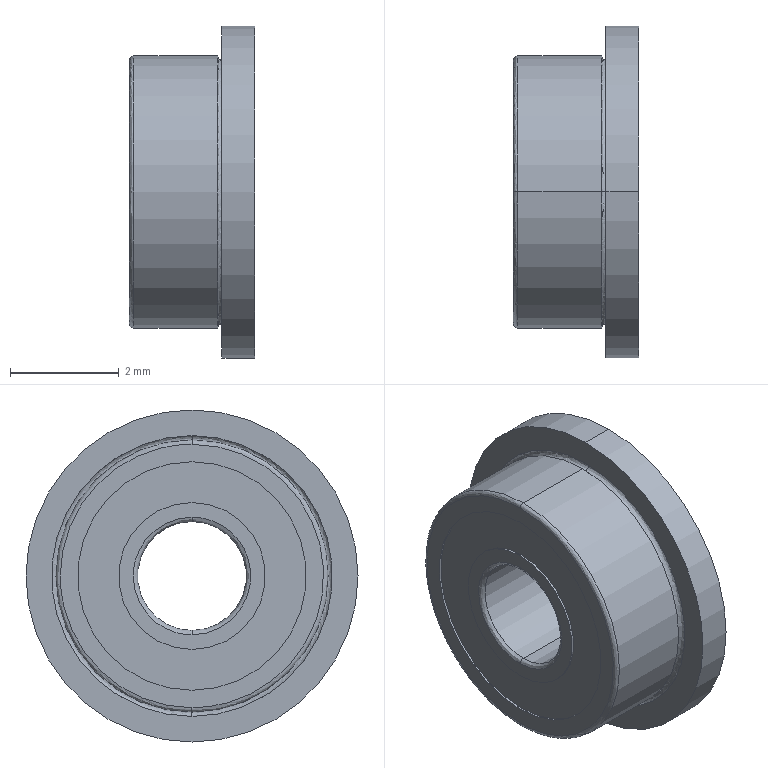Part | SolidWorks | features BaseBody 1 | 1 solid | 29 faces | box 2.3 x 6.1 x 6.1 mm | volume 42.794 mm3 | cylinder 14 | spline 8 | plane 7 | commonest cylinder face diameters 2.7 x4 4.2 x4 2 x2 5 x2 6.1 x2
STEP:
#1=CARTESIAN_POINT('',(1.7,0.,-2.58));
#2=VERTEX_POINT('',#1);
#3=CARTESIAN_POINT('',(1.7,0.,2.58));
#4=VERTEX_POINT('',#3);
#5=CARTESIAN_POINT('',(1.7,0.,0.));
#6=DIRECTION('',(1.,0.,0.));
#7=DIRECTION('',(0.,0.,1.));
#8=AXIS2_PLACEMENT_3D('',#5,#6,#7);
#9=CIRCLE('',#8,2.58);
#10=EDGE_CURVE('',#2,#4,#9,.T.);
#11=ORIENTED_EDGE('',*,*,#10,.F.);
#12=CARTESIAN_POINT('',(1.62,0.,-2.5));
#13=VERTEX_POINT('',#12);
#14=CARTESIAN_POINT('',(1.7,0.,-2.5));
#15=DIRECTION('',(0.,-1.,0.));
#16=DIRECTION('',(0.,0.,-1.));
#17=AXIS2_PLACEMENT_3D('',#14,#15,#16);
#18=CIRCLE('',#17,0.08);
#19=EDGE_CURVE('',#2,#13,#18,.T.);
#20=ORIENTED_EDGE('',*,*,#19,.T.);
#21=CARTESIAN_POINT('',(1.62,0.,2.5));
#22=VERTEX_POINT('',#21);
#23=CARTESIAN_POINT('',(1.62,0.,0.));
#24=DIRECTION('',(-1.,0.,0.));
#25=DIRECTION('',(0.,0.,1.));
#26=AXIS2_PLACEMENT_3D('',#23,#24,#25);
#27=CIRCLE('',#26,2.5);
#28=EDGE_CURVE('',#22,#13,#27,.T.);
#29=ORIENTED_EDGE('',*,*,#28,.F.);
#30=CARTESIAN_POINT('',(1.7,0.,2.5));
#31=DIRECTION('',(0.,1.,0.));
#32=DIRECTION('',(0.,0.,1.));
#33=AXIS2_PLACEMENT_3D('',#30,#31,#32);
#34=CIRCLE('',#33,0.08);
#35=EDGE_CURVE('',#4,#22,#34,.T.);
#36=ORIENTED_EDGE('',*,*,#35,.F.);
#37=EDGE_LOOP('',(#11,#20,#29,#36));
#38=FACE_OUTER_BOUND('',#37,.T.);
#39=CARTESIAN_POINT('',(1.7,0.,2.58));
#40=CARTESIAN_POINT('',(1.7,5.16,2.58));
#41=CARTESIAN_POINT('',(1.7,5.16,-2.58));
#42=CARTESIAN_POINT('',(1.7,0.,-2.58));
#43=CARTESIAN_POINT('',(1.784,0.,2.58));
#44=CARTESIAN_POINT('',(1.784,5.16,2.58));
#45=CARTESIAN_POINT('',(1.784,5.16,-2.58));
#46=CARTESIAN_POINT('',(1.784,0.,-2.58));
#47=CARTESIAN_POINT('',(1.816,0.,2.503));
#48=CARTESIAN_POINT('',(1.816,5.005,2.503));
#49=CARTESIAN_POINT('',(1.816,5.005,-2.503));
#50=CARTESIAN_POINT('',(1.816,0.,-2.503));
#51=CARTESIAN_POINT('',(1.757,0.,2.443));
#52=CARTESIAN_POINT('',(1.757,4.887,2.443));
#53=CARTESIAN_POINT('',(1.757,4.887,-2.443));
#54=CARTESIAN_POINT('',(1.757,0.,-2.443));
#55=CARTESIAN_POINT('',(1.697,0.,2.384));
#56=CARTESIAN_POINT('',(1.697,4.768,2.384));
#57=CARTESIAN_POINT('',(1.697,4.768,-2.384));
#58=CARTESIAN_POINT('',(1.697,0.,-2.384));
#59=CARTESIAN_POINT('',(1.62,0.,2.416));
#60=CARTESIAN_POINT('',(1.62,4.833,2.416));
#61=CARTESIAN_POINT('',(1.62,4.833,-2.416));
#62=CARTESIAN_POINT('',(1.62,0.,-2.416));
#63=CARTESIAN_POINT('',(1.62,0.,2.5));
#64=CARTESIAN_POINT('',(1.62,5.,2.5));
#65=CARTESIAN_POINT('',(1.62,5.,-2.5));
#66=CARTESIAN_POINT('',(1.62,0.,-2.5));
#67=(BOUNDED_SURFACE()B_SPLINE_SURFACE(3,3,((#39,#40,#41,#42),(#43,#44,#45,#46),(#47,#48,#49,#50),(#51,#52,#53,#54),(#55,#56,#57,#58),(#59,#60,#61,#62),(#63,#64,#65,#66)),.UNSPECIFIED.,.F.,.F.,.T.)B_SPLINE_SURFACE_WITH_KNOTS((4,3,4),(4,4),(0.,0.5,1.),(0.,1.),.UNSPECIFIED.)GEOMETRIC_REPRESENTATION_ITEM()RATIONAL_B_SPLINE_SURFACE(((1.,0.3333,0.3333,1.),(0.5885,0.1962,0.1962,0.5885),(0.5885,0.1962,0.1962,0.5885),(1.,0.3333,0.3333,1.),(0.5885,0.1962,0.1962,0.5885),(0.5885,0.1962,0.1962,0.5885),(1.,0.3333,0.3333,1.)))REPRESENTATION_ITEM('')SURFACE());
#68=ADVANCED_FACE('',(#38),#67,.F.);
#69=CARTESIAN_POINT('',(2.3,0.,-1.08));
#70=VERTEX_POINT('',#69);
#71=CARTESIAN_POINT('',(2.3,0.,1.08));
#72=VERTEX_POINT('',#71);
#73=CARTESIAN_POINT('',(2.3,0.,-1.08));
#74=CARTESIAN_POINT('',(2.3,-0.06875,-1.08));
#75=CARTESIAN_POINT('',(2.3,-0.17,-1.07));
#76=CARTESIAN_POINT('',(2.3,-0.2849,-1.043));
#77=CARTESIAN_POINT('',(2.3,-0.3334,-1.027));
#78=CARTESIAN_POINT('',(2.3,-0.3656,-1.016));
#79=CARTESIAN_POINT('',(2.3,-0.3802,-1.011));
#80=CARTESIAN_POINT('',(2.3,-0.5359,-0.9495));
#81=CARTESIAN_POINT('',(2.3,-0.6584,-0.8688));
#82=CARTESIAN_POINT('',(2.3,-0.8163,-0.7111));
#83=CARTESIAN_POINT('',(2.3,-0.8858,-0.6259));
#84=CARTESIAN_POINT('',(2.3,-0.9505,-0.5154));
#85=CARTESIAN_POINT('',(2.3,-0.9747,-0.4657));
#86=CARTESIAN_POINT('',(2.3,-0.99,-0.432));
#87=CARTESIAN_POINT('',(2.3,-0.9979,-0.4135));
#88=CARTESIAN_POINT('',(2.3,-1.055,-0.2702));
#89=CARTESIAN_POINT('',(2.3,-1.08,-0.137));
#90=CARTESIAN_POINT('',(2.3,-1.08,0.06849));
#91=CARTESIAN_POINT('',(2.3,-1.071,0.1696));
#92=CARTESIAN_POINT('',(2.3,-1.043,0.2845));
#93=CARTESIAN_POINT('',(2.3,-1.028,0.3332));
#94=CARTESIAN_POINT('',(2.3,-1.016,0.3655));
#95=CARTESIAN_POINT('',(2.3,-1.011,0.3802));
#96=CARTESIAN_POINT('',(2.3,-0.9495,0.5359));
#97=CARTESIAN_POINT('',(2.3,-0.8688,0.6584));
#98=CARTESIAN_POINT('',(2.3,-0.7111,0.8163));
#99=CARTESIAN_POINT('',(2.3,-0.6259,0.8858));
#100=CARTESIAN_POINT('',(2.3,-0.5154,0.9505));
#101=CARTESIAN_POINT('',(2.3,-0.4657,0.9747));
#102=CARTESIAN_POINT('',(2.3,-0.432,0.99));
#103=CARTESIAN_POINT('',(2.3,-0.4134,0.9979));
#104=CARTESIAN_POINT('',(2.3,-0.2704,1.055));
#105=CARTESIAN_POINT('',(2.3,-0.1379,1.08));
#106=CARTESIAN_POINT('',(2.3,0.,1.08));
#107=B_SPLINE_CURVE_WITH_KNOTS('',3,(#73,#74,#75,#76,#77,#78,#79,#80,#81,#82,#83,#84,#85,#86,#87,#88,#89,#90,#91,#92,#93,#94,#95,#96,#97,#98,#99,#100,#101,#102,#103,#104,#105,#106),.UNSPECIFIED.,.F.,.F.,(4,1,1,2,2,2,1,1,2,2,2,1,1,2,2,2,1,1,2,2,4),(0.,0.0625,0.09375,0.1094,0.125,0.25,0.3125,0.3438,0.3594,0.375,0.5,0.5625,0.5938,0.6094,0.625,0.75,0.8125,0.8438,0.8594,0.875,1.),.UNSPECIFIED.);
#108=EDGE_CURVE('',#70,#72,#107,.T.);
#109=ORIENTED_EDGE('',*,*,#108,.F.);
#110=CARTESIAN_POINT('',(2.22,0.,-1.));
#111=VERTEX_POINT('',#110);
#112=CARTESIAN_POINT('',(2.22,0.,-1.08));
#113=DIRECTION('',(0.,-1.,0.));
#114=DIRECTION('',(0.,0.,-1.));
#115=AXIS2_PLACEMENT_3D('',#112,#113,#114);
#116=CIRCLE('',#115,0.08);
#117=EDGE_CURVE('',#70,#111,#116,.T.);
#118=ORIENTED_EDGE('',*,*,#117,.T.);
#119=CARTESIAN_POINT('',(2.22,0.,1.));
#120=VERTEX_POINT('',#119);
#121=CARTESIAN_POINT('',(2.22,0.,0.));
#122=DIRECTION('',(-1.,0.,0.));
#123=DIRECTION('',(0.,0.,1.));
#124=AXIS2_PLACEMENT_3D('',#121,#122,#123);
#125=CIRCLE('',#124,1.);
#126=EDGE_CURVE('',#111,#120,#125,.T.);
#127=ORIENTED_EDGE('',*,*,#126,.T.);
#128=CARTESIAN_POINT('',(2.22,0.,1.08));
#129=DIRECTION('',(0.,1.,0.));
#130=DIRECTION('',(0.,0.,1.));
#131=AXIS2_PLACEMENT_3D('',#128,#129,#130);
#132=CIRCLE('',#131,0.08);
#133=EDGE_CURVE('',#72,#120,#132,.T.);
#134=ORIENTED_EDGE('',*,*,#133,.F.);
#135=EDGE_LOOP('',(#109,#118,#127,#134));
#136=FACE_OUTER_BOUND('',#135,.T.);
#137=CARTESIAN_POINT('',(2.3,0.,-1.08));
#138=CARTESIAN_POINT('',(2.3,-2.16,-1.08));
#139=CARTESIAN_POINT('',(2.3,-2.16,1.08));
#140=CARTESIAN_POINT('',(2.3,0.,1.08));
#141=CARTESIAN_POINT('',(2.3,0.,-1.033));
#142=CARTESIAN_POINT('',(2.3,-2.066,-1.033));
#143=CARTESIAN_POINT('',(2.3,-2.066,1.033));
#144=CARTESIAN_POINT('',(2.3,0.,1.033));
#145=CARTESIAN_POINT('',(2.267,0.,-1.));
#146=CARTESIAN_POINT('',(2.267,-2.,-1.));
#147=CARTESIAN_POINT('',(2.267,-2.,1.));
#148=CARTESIAN_POINT('',(2.267,0.,1.));
#149=CARTESIAN_POINT('',(2.22,0.,-1.));
#150=CARTESIAN_POINT('',(2.22,-2.,-1.));
#151=CARTESIAN_POINT('',(2.22,-2.,1.));
#152=CARTESIAN_POINT('',(2.22,0.,1.));
#153=(BOUNDED_SURFACE()B_SPLINE_SURFACE(3,3,((#137,#138,#139,#140),(#141,#142,#143,#144),(#145,#146,#147,#148),(#149,#150,#151,#152)),.UNSPECIFIED.,.F.,.F.,.T.)B_SPLINE_SURFACE_WITH_KNOTS((4,4),(4,4),(0.,1.),(0.,1.),.UNSPECIFIED.)GEOMETRIC_REPRESENTATION_ITEM()RATIONAL_B_SPLINE_SURFACE(((1.,0.3333,0.3333,1.),(0.8047,0.2682,0.2682,0.8047),(0.8047,0.2682,0.2682,0.8047),(1.,0.3333,0.3333,1.)))REPRESENTATION_ITEM('')SURFACE());
#154=ADVANCED_FACE('',(#136),#153,.T.);
#155=CARTESIAN_POINT('',(0.,0.,2.42));
#156=VERTEX_POINT('',#155);
#157=CARTESIAN_POINT('',(0.,0.,-2.42));
#158=VERTEX_POINT('',#157);
#159=CARTESIAN_POINT('',(0.,0.,2.42));
#160=CARTESIAN_POINT('',(0.,-4.84,2.42));
#161=CARTESIAN_POINT('',(0.,-4.84,-2.42));
#162=CARTESIAN_POINT('',(0.,0.,-2.42));
#163=(BOUNDED_CURVE()B_SPLINE_CURVE(3,(#159,#160,#161,#162),.UNSPECIFIED.,.F.,.F.)B_SPLINE_CURVE_WITH_KNOTS((4,4),(0.,1.),.UNSPECIFIED.)CURVE()GEOMETRIC_REPRESENTATION_ITEM()RATIONAL_B_SPLINE_CURVE((1.,0.3333,0.3333,1.))REPRESENTATION_ITEM(''));
#164=EDGE_CURVE('',#156,#158,#163,.T.);
#165=ORIENTED_EDGE('',*,*,#164,.T.);
#166=CARTESIAN_POINT('',(0.08,0.,-2.5));
#167=VERTEX_POINT('',#166);
#168=CARTESIAN_POINT('',(0.08,0.,-2.42));
#169=DIRECTION('',(0.,-1.,0.));
#170=DIRECTION('',(0.,0.,-1.));
#171=AXIS2_PLACEMENT_3D('',#168,#169,#170);
#172=CIRCLE('',#171,0.08);
#173=EDGE_CURVE('',#158,#167,#172,.T.);
#174=ORIENTED_EDGE('',*,*,#173,.T.);
#175=CARTESIAN_POINT('',(0.08,0.,2.5));
#176=VERTEX_POINT('',#175);
#177=CARTESIAN_POINT('',(0.08,0.,0.));
#178=DIRECTION('',(1.,0.,0.));
#179=DIRECTION('',(0.,0.,-1.));
#180=AXIS2_PLACEMENT_3D('',#177,#178,#179);
#181=CIRCLE('',#180,2.5);
#182=EDGE_CURVE('',#176,#167,#181,.T.);
#183=ORIENTED_EDGE('',*,*,#182,.F.);
#184=CARTESIAN_POINT('',(0.08,0.,2.42));
#185=DIRECTION('',(0.,1.,0.));
#186=DIRECTION('',(0.,0.,1.));
#187=AXIS2_PLACEMENT_3D('',#184,#185,#186);
#188=CIRCLE('',#187,0.08);
#189=EDGE_CURVE('',#156,#176,#188,.T.);
#190=ORIENTED_EDGE('',*,*,#189,.F.);
#191=EDGE_LOOP('',(#165,#174,#183,#190));
#192=FACE_OUTER_BOUND('',#191,.T.);
#193=CARTESIAN_POINT('',(0.,0.,-2.42));
#194=CARTESIAN_POINT('',(0.,-4.84,-2.42));
#195=CARTESIAN_POINT('',(0.,-4.84,2.42));
#196=CARTESIAN_POINT('',(0.,0.,2.42));
#197=CARTESIAN_POINT('',(0.,0.,-2.467));
#198=CARTESIAN_POINT('',(0.,-4.934,-2.467));
#199=CARTESIAN_POINT('',(0.,-4.934,2.467));
#200=CARTESIAN_POINT('',(0.,0.,2.467));
#201=CARTESIAN_POINT('',(0.03314,0.,-2.5));
#202=CARTESIAN_POINT('',(0.03314,-5.,-2.5));
#203=CARTESIAN_POINT('',(0.03314,-5.,2.5));
#204=CARTESIAN_POINT('',(0.03314,0.,2.5));
#205=CARTESIAN_POINT('',(0.08,0.,-2.5));
#206=CARTESIAN_POINT('',(0.08,-5.,-2.5));
#207=CARTESIAN_POINT('',(0.08,-5.,2.5));
#208=CARTESIAN_POINT('',(0.08,0.,2.5));
#209=(BOUNDED_SURFACE()B_SPLINE_SURFACE(3,3,((#193,#194,#195,#196),(#197,#198,#199,#200),(#201,#202,#203,#204),(#205,#206,#207,#208)),.UNSPECIFIED.,.F.,.F.,.T.)B_SPLINE_SURFACE_WITH_KNOTS((4,4),(4,4),(0.,1.),(0.,1.),.UNSPECIFIED.)GEOMETRIC_REPRESENTATION_ITEM()RATIONAL_B_SPLINE_SURFACE(((1.,0.3333,0.3333,1.),(0.8047,0.2682,0.2682,0.8047),(0.8047,0.2682,0.2682,0.8047),(1.,0.3333,0.3333,1.)))REPRESENTATION_ITEM('')SURFACE());
#210=ADVANCED_FACE('',(#192),#209,.T.);
#211=CARTESIAN_POINT('',(0.08,0.,1.));
#212=VERTEX_POINT('',#211);
#213=CARTESIAN_POINT('',(0.08,0.,-1.));
#214=VERTEX_POINT('',#213);
#215=CARTESIAN_POINT('',(0.08,0.,0.));
#216=DIRECTION('',(1.,0.,0.));
#217=DIRECTION('',(0.,0.,-1.));
#218=AXIS2_PLACEMENT_3D('',#215,#216,#217);
#219=CIRCLE('',#218,1.);
#220=EDGE_CURVE('',#212,#214,#219,.T.);
#221=ORIENTED_EDGE('',*,*,#220,.T.);
#222=CARTESIAN_POINT('',(0.,0.,-1.08));
#223=VERTEX_POINT('',#222);
#224=CARTESIAN_POINT('',(0.08,0.,-1.08));
#225=DIRECTION('',(0.,-1.,0.));
#226=DIRECTION('',(0.,0.,-1.));
#227=AXIS2_PLACEMENT_3D('',#224,#225,#226);
#228=CIRCLE('',#227,0.08);
#229=EDGE_CURVE('',#214,#223,#228,.T.);
#230=ORIENTED_EDGE('',*,*,#229,.T.);
#231=CARTESIAN_POINT('',(0.,0.,1.08));
#232=VERTEX_POINT('',#231);
#233=CARTESIAN_POINT('',(0.,0.,-1.08));
#234=CARTESIAN_POINT('',(0.,-2.16,-1.08));
#235=CARTESIAN_POINT('',(0.,-2.16,1.08));
#236=CARTESIAN_POINT('',(0.,0.,1.08));
#237=(BOUNDED_CURVE()B_SPLINE_CURVE(3,(#233,#234,#235,#236),.UNSPECIFIED.,.F.,.T.)B_SPLINE_CURVE_WITH_KNOTS((4,4),(0.,1.),.UNSPECIFIED.)CURVE()GEOMETRIC_REPRESENTATION_ITEM()RATIONAL_B_SPLINE_CURVE((1.,0.3333,0.3333,1.))REPRESENTATION_ITEM(''));
#238=EDGE_CURVE('',#223,#232,#237,.T.);
#239=ORIENTED_EDGE('',*,*,#238,.T.);
#240=CARTESIAN_POINT('',(0.08,0.,1.08));
#241=DIRECTION('',(0.,1.,0.));
#242=DIRECTION('',(0.,0.,1.));
#243=AXIS2_PLACEMENT_3D('',#240,#241,#242);
#244=CIRCLE('',#243,0.08);
#245=EDGE_CURVE('',#212,#232,#244,.T.);
#246=ORIENTED_EDGE('',*,*,#245,.F.);
#247=EDGE_LOOP('',(#221,#230,#239,#246));
#248=FACE_OUTER_BOUND('',#247,.T.);
#249=CARTESIAN_POINT('',(0.08,0.,-1.));
#250=CARTESIAN_POINT('',(0.08,-2.,-1.));
#251=CARTESIAN_POINT('',(0.08,-2.,1.));
#252=CARTESIAN_POINT('',(0.08,0.,1.));
#253=CARTESIAN_POINT('',(0.03314,0.,-1.));
#254=CARTESIAN_POINT('',(0.03314,-2.,-1.));
#255=CARTESIAN_POINT('',(0.03314,-2.,1.));
#256=CARTESIAN_POINT('',(0.03314,0.,1.));
#257=CARTESIAN_POINT('',(0.,0.,-1.033));
#258=CARTESIAN_POINT('',(0.,-2.066,-1.033));
#259=CARTESIAN_POINT('',(0.,-2.066,1.033));
#260=CARTESIAN_POINT('',(0.,0.,1.033));
#261=CARTESIAN_POINT('',(0.,0.,-1.08));
#262=CARTESIAN_POINT('',(0.,-2.16,-1.08));
#263=CARTESIAN_POINT('',(0.,-2.16,1.08));
#264=CARTESIAN_POINT('',(0.,0.,1.08));
#265=(BOUNDED_SURFACE()B_SPLINE_SURFACE(3,3,((#249,#250,#251,#252),(#253,#254,#255,#256),(#257,#258,#259,#260),(#261,#262,#263,#264)),.UNSPECIFIED.,.F.,.F.,.T.)B_SPLINE_SURFACE_WITH_KNOTS((4,4),(4,4),(0.,1.),(0.,1.),.UNSPECIFIED.)GEOMETRIC_REPRESENTATION_ITEM()RATIONAL_B_SPLINE_SURFACE(((1.,0.3333,0.3333,1.),(0.8047,0.2682,0.2682,0.8047),(0.8047,0.2682,0.2682,0.8047),(1.,0.3333,0.3333,1.)))REPRESENTATION_ITEM('')SURFACE());
#266=ADVANCED_FACE('',(#248),#265,.T.);
#267=CARTESIAN_POINT('',(2.262,0.,2.1));
#268=VERTEX_POINT('',#267);
#269=CARTESIAN_POINT('',(2.262,0.,-2.1));
#270=VERTEX_POINT('',#269);
#271=CARTESIAN_POINT('',(2.262,0.,0.));
#272=DIRECTION('',(1.,0.,0.));
#273=DIRECTION('',(0.,0.,-1.));
#274=AXIS2_PLACEMENT_3D('',#271,#272,#273);
#275=CIRCLE('',#274,2.1);
#276=EDGE_CURVE('',#268,#270,#275,.T.);
#277=ORIENTED_EDGE('',*,*,#276,.F.);
#278=CARTESIAN_POINT('',(2.3,0.,2.1));
#279=VERTEX_POINT('',#278);
#280=CARTESIAN_POINT('',(2.281,0.,2.1));
#281=DIRECTION('',(1.,0.,0.));
#282=VECTOR('',#281,1000.);
#283=LINE('',#280,#282);
#284=EDGE_CURVE('',#268,#279,#283,.T.);
#285=ORIENTED_EDGE('',*,*,#284,.T.);
#286=CARTESIAN_POINT('',(2.3,0.,-2.1));
#287=VERTEX_POINT('',#286);
#288=CARTESIAN_POINT('',(2.3,0.,0.));
#289=DIRECTION('',(-1.,0.,0.));
#290=DIRECTION('',(0.,0.,-1.));
#291=AXIS2_PLACEMENT_3D('',#288,#289,#290);
#292=CIRCLE('',#291,2.1);
#293=EDGE_CURVE('',#287,#279,#292,.T.);
#294=ORIENTED_EDGE('',*,*,#293,.F.);
#295=CARTESIAN_POINT('',(2.281,0.,-2.1));
#296=DIRECTION('',(1.,0.,0.));
#297=VECTOR('',#296,1000.);
#298=LINE('',#295,#297);
#299=EDGE_CURVE('',#270,#287,#298,.T.);
#300=ORIENTED_EDGE('',*,*,#299,.F.);
#301=EDGE_LOOP('',(#277,#285,#294,#300));
#302=FACE_OUTER_BOUND('',#301,.T.);
#303=CARTESIAN_POINT('',(2.281,0.,0.));
#304=DIRECTION('',(1.,0.,0.));
#305=DIRECTION('',(0.,0.,-1.));
#306=AXIS2_PLACEMENT_3D('',#303,#304,#305);
#307=CYLINDRICAL_SURFACE('',#306,2.1);
#308=ADVANCED_FACE('',(#302),#307,.F.);
#309=CARTESIAN_POINT('',(1.7,0.,-3.05));
#310=VERTEX_POINT('',#309);
#311=CARTESIAN_POINT('',(1.7,0.,3.05));
#312=VERTEX_POINT('',#311);
#313=CARTESIAN_POINT('',(1.7,0.,0.));
#314=DIRECTION('',(1.,0.,0.));
#315=DIRECTION('',(0.,0.,-1.));
#316=AXIS2_PLACEMENT_3D('',#313,#314,#315);
#317=CIRCLE('',#316,3.05);
#318=EDGE_CURVE('',#310,#312,#317,.T.);
#319=ORIENTED_EDGE('',*,*,#318,.T.);
#320=CARTESIAN_POINT('',(2.3,0.,3.05));
#321=VERTEX_POINT('',#320);
#322=CARTESIAN_POINT('',(2.,0.,3.05));
#323=DIRECTION('',(1.,0.,0.));
#324=VECTOR('',#323,1000.);
#325=LINE('',#322,#324);
#326=EDGE_CURVE('',#312,#321,#325,.T.);
#327=ORIENTED_EDGE('',*,*,#326,.T.);
#328=CARTESIAN_POINT('',(2.3,0.,-3.05));
#329=VERTEX_POINT('',#328);
#330=CARTESIAN_POINT('',(2.3,0.,0.));
#331=DIRECTION('',(1.,0.,0.));
#332=DIRECTION('',(0.,0.,-1.));
#333=AXIS2_PLACEMENT_3D('',#330,#331,#332);
#334=CIRCLE('',#333,3.05);
#335=EDGE_CURVE('',#329,#321,#334,.T.);
#336=ORIENTED_EDGE('',*,*,#335,.F.);
#337=CARTESIAN_POINT('',(2.,0.,-3.05));
#338=DIRECTION('',(1.,0.,0.));
#339=VECTOR('',#338,1000.);
#340=LINE('',#337,#339);
#341=EDGE_CURVE('',#310,#329,#340,.T.);
#342=ORIENTED_EDGE('',*,*,#341,.F.);
#343=EDGE_LOOP('',(#319,#327,#336,#342));
#344=FACE_OUTER_BOUND('',#343,.T.);
#345=CARTESIAN_POINT('',(2.,0.,0.));
#346=DIRECTION('',(1.,0.,0.));
#347=DIRECTION('',(0.,0.,-1.));
#348=AXIS2_PLACEMENT_3D('',#345,#346,#347);
#349=CYLINDRICAL_SURFACE('',#348,3.05);
#350=ADVANCED_FACE('',(#344),#349,.T.);
#351=CARTESIAN_POINT('',(2.262,0.,1.35));
#352=VERTEX_POINT('',#351);
#353=CARTESIAN_POINT('',(2.262,0.,-1.35));
#354=VERTEX_POINT('',#353);
#355=CARTESIAN_POINT('',(2.262,0.,0.));
#356=DIRECTION('',(-1.,0.,0.));
#357=DIRECTION('',(0.,0.,-1.));
#358=AXIS2_PLACEMENT_3D('',#355,#356,#357);
#359=CIRCLE('',#358,1.35);
#360=EDGE_CURVE('',#352,#354,#359,.T.);
#361=ORIENTED_EDGE('',*,*,#360,.F.);
#362=CARTESIAN_POINT('',(2.3,0.,1.35));
#363=VERTEX_POINT('',#362);
#364=CARTESIAN_POINT('',(2.281,0.,1.35));
#365=DIRECTION('',(1.,0.,0.));
#366=VECTOR('',#365,1000.);
#367=LINE('',#364,#366);
#368=EDGE_CURVE('',#352,#363,#367,.T.);
#369=ORIENTED_EDGE('',*,*,#368,.T.);
#370=CARTESIAN_POINT('',(2.3,0.,-1.35));
#371=VERTEX_POINT('',#370);
#372=CARTESIAN_POINT('',(2.3,0.,0.));
#373=DIRECTION('',(-1.,0.,0.));
#374=DIRECTION('',(0.,0.,-1.));
#375=AXIS2_PLACEMENT_3D('',#372,#373,#374);
#376=CIRCLE('',#375,1.35);
#377=EDGE_CURVE('',#363,#371,#376,.T.);
#378=ORIENTED_EDGE('',*,*,#377,.T.);
#379=CARTESIAN_POINT('',(2.281,0.,-1.35));
#380=DIRECTION('',(1.,0.,0.));
#381=VECTOR('',#380,1000.);
#382=LINE('',#379,#381);
#383=EDGE_CURVE('',#354,#371,#382,.T.);
#384=ORIENTED_EDGE('',*,*,#383,.F.);
#385=EDGE_LOOP('',(#361,#369,#378,#384));
#386=FACE_OUTER_BOUND('',#385,.T.);
#387=CARTESIAN_POINT('',(2.281,0.,0.));
#388=DIRECTION('',(1.,0.,0.));
#389=DIRECTION('',(0.,0.,-1.));
#390=AXIS2_PLACEMENT_3D('',#387,#388,#389);
#391=CYLINDRICAL_SURFACE('',#390,1.35);
#392=ADVANCED_FACE('',(#386),#391,.T.);
#393=CARTESIAN_POINT('',(0.08,0.,0.));
#394=DIRECTION('',(1.,0.,0.));
#395=DIRECTION('',(0.,0.,-1.));
#396=AXIS2_PLACEMENT_3D('',#393,#394,#395);
#397=CIRCLE('',#396,2.5);
#398=EDGE_CURVE('',#167,#176,#397,.T.);
#399=ORIENTED_EDGE('',*,*,#398,.T.);
#400=CARTESIAN_POINT('',(0.85,0.,2.5));
#401=DIRECTION('',(1.,0.,0.));
#402=VECTOR('',#401,1000.);
#403=LINE('',#400,#402);
#404=EDGE_CURVE('',#176,#22,#403,.T.);
#405=ORIENTED_EDGE('',*,*,#404,.T.);
#406=ORIENTED_EDGE('',*,*,#28,.T.);
#407=CARTESIAN_POINT('',(0.85,0.,-2.5));
#408=DIRECTION('',(1.,0.,0.));
#409=VECTOR('',#408,1000.);
#410=LINE('',#407,#409);
#411=EDGE_CURVE('',#167,#13,#410,.T.);
#412=ORIENTED_EDGE('',*,*,#411,.F.);
#413=EDGE_LOOP('',(#399,#405,#406,#412));
#414=FACE_OUTER_BOUND('',#413,.T.);
#415=CARTESIAN_POINT('',(0.85,0.,0.));
#416=DIRECTION('',(1.,0.,0.));
#417=DIRECTION('',(0.,0.,-1.));
#418=AXIS2_PLACEMENT_3D('',#415,#416,#417);
#419=CYLINDRICAL_SURFACE('',#418,2.5);
#420=ADVANCED_FACE('',(#414),#419,.T.);
#421=ORIENTED_EDGE('',*,*,#220,.F.);
#422=CARTESIAN_POINT('',(1.15,0.,1.));
#423=DIRECTION('',(1.,0.,0.));
#424=VECTOR('',#423,1000.);
#425=LINE('',#422,#424);
#426=EDGE_CURVE('',#212,#120,#425,.T.);
#427=ORIENTED_EDGE('',*,*,#426,.T.);
#428=ORIENTED_EDGE('',*,*,#126,.F.);
#429=CARTESIAN_POINT('',(1.15,0.,-1.));
#430=DIRECTION('',(1.,0.,0.));
#431=VECTOR('',#430,1000.);
#432=LINE('',#429,#431);
#433=EDGE_CURVE('',#214,#111,#432,.T.);
#434=ORIENTED_EDGE('',*,*,#433,.F.);
#435=EDGE_LOOP('',(#421,#427,#428,#434));
#436=FACE_OUTER_BOUND('',#435,.T.);
#437=CARTESIAN_POINT('',(1.15,0.,0.));
#438=DIRECTION('',(1.,0.,0.));
#439=DIRECTION('',(0.,0.,-1.));
#440=AXIS2_PLACEMENT_3D('',#437,#438,#439);
#441=CYLINDRICAL_SURFACE('',#440,1.);
#442=ADVANCED_FACE('',(#436),#441,.F.);
#443=CARTESIAN_POINT('',(0.,0.,2.1));
#444=VERTEX_POINT('',#443);
#445=CARTESIAN_POINT('',(0.,0.,-2.1));
#446=VERTEX_POINT('',#445);
#447=CARTESIAN_POINT('',(0.,0.,0.));
#448=DIRECTION('',(1.,0.,0.));
#449=DIRECTION('',(0.,0.,-1.));
#450=AXIS2_PLACEMENT_3D('',#447,#448,#449);
#451=CIRCLE('',#450,2.1);
#452=EDGE_CURVE('',#444,#446,#451,.T.);
#453=ORIENTED_EDGE('',*,*,#452,.F.);
#454=CARTESIAN_POINT('',(0.0382,0.,2.1));
#455=VERTEX_POINT('',#454);
#456=CARTESIAN_POINT('',(0.0191,0.,2.1));
#457=DIRECTION('',(1.,0.,0.));
#458=VECTOR('',#457,1000.);
#459=LINE('',#456,#458);
#460=EDGE_CURVE('',#444,#455,#459,.T.);
#461=ORIENTED_EDGE('',*,*,#460,.T.);
#462=CARTESIAN_POINT('',(0.0382,0.,-2.1));
#463=VERTEX_POINT('',#462);
#464=CARTESIAN_POINT('',(0.0382,0.,0.));
#465=DIRECTION('',(-1.,0.,0.));
#466=DIRECTION('',(0.,0.,-1.));
#467=AXIS2_PLACEMENT_3D('',#464,#465,#466);
#468=CIRCLE('',#467,2.1);
#469=EDGE_CURVE('',#463,#455,#468,.T.);
#470=ORIENTED_EDGE('',*,*,#469,.F.);
#471=CARTESIAN_POINT('',(0.0191,0.,-2.1));
#472=DIRECTION('',(1.,0.,0.));
#473=VECTOR('',#472,1000.);
#474=LINE('',#471,#473);
#475=EDGE_CURVE('',#446,#463,#474,.T.);
#476=ORIENTED_EDGE('',*,*,#475,.F.);
#477=EDGE_LOOP('',(#453,#461,#470,#476));
#478=FACE_OUTER_BOUND('',#477,.T.);
#479=CARTESIAN_POINT('',(0.0191,0.,0.));
#480=DIRECTION('',(1.,0.,0.));
#481=DIRECTION('',(0.,0.,-1.));
#482=AXIS2_PLACEMENT_3D('',#479,#480,#481);
#483=CYLINDRICAL_SURFACE('',#482,2.1);
#484=ADVANCED_FACE('',(#478),#483,.F.);
#485=CARTESIAN_POINT('',(0.,0.,1.35));
#486=VERTEX_POINT('',#485);
#487=CARTESIAN_POINT('',(0.,0.,-1.35));
#488=VERTEX_POINT('',#487);
#489=CARTESIAN_POINT('',(0.,0.,0.));
#490=DIRECTION('',(-1.,0.,0.));
#491=DIRECTION('',(0.,0.,-1.));
#492=AXIS2_PLACEMENT_3D('',#489,#490,#491);
#493=CIRCLE('',#492,1.35);
#494=EDGE_CURVE('',#486,#488,#493,.T.);
#495=ORIENTED_EDGE('',*,*,#494,.F.);
#496=CARTESIAN_POINT('',(0.0382,0.,1.35));
#497=VERTEX_POINT('',#496);
#498=CARTESIAN_POINT('',(0.0191,0.,1.35));
#499=DIRECTION('',(1.,0.,0.));
#500=VECTOR('',#499,1000.);
#501=LINE('',#498,#500);
#502=EDGE_CURVE('',#486,#497,#501,.T.);
#503=ORIENTED_EDGE('',*,*,#502,.T.);
#504=CARTESIAN_POINT('',(0.0382,0.,-1.35));
#505=VERTEX_POINT('',#504);
#506=CARTESIAN_POINT('',(0.0382,0.,0.));
#507=DIRECTION('',(-1.,0.,0.));
#508=DIRECTION('',(0.,0.,-1.));
#509=AXIS2_PLACEMENT_3D('',#506,#507,#508);
#510=CIRCLE('',#509,1.35);
#511=EDGE_CURVE('',#497,#505,#510,.T.);
#512=ORIENTED_EDGE('',*,*,#511,.T.);
#513=CARTESIAN_POINT('',(0.0191,0.,-1.35));
#514=DIRECTION('',(1.,0.,0.));
#515=VECTOR('',#514,1000.);
#516=LINE('',#513,#515);
#517=EDGE_CURVE('',#488,#505,#516,.T.);
#518=ORIENTED_EDGE('',*,*,#517,.F.);
#519=EDGE_LOOP('',(#495,#503,#512,#518));
#520=FACE_OUTER_BOUND('',#519,.T.);
#521=CARTESIAN_POINT('',(0.0191,0.,0.));
#522=DIRECTION('',(1.,0.,0.));
#523=DIRECTION('',(0.,0.,-1.));
#524=AXIS2_PLACEMENT_3D('',#521,#522,#523);
#525=CYLINDRICAL_SURFACE('',#524,1.35);
#526=ADVANCED_FACE('',(#520),#525,.T.);
#527=ORIENTED_EDGE('',*,*,#293,.T.);
#528=CARTESIAN_POINT('',(2.3,0.,0.));
#529=DIRECTION('',(-1.,0.,0.));
#530=DIRECTION('',(0.,0.,-1.));
#531=AXIS2_PLACEMENT_3D('',#528,#529,#530);
#532=CIRCLE('',#531,2.1);
#533=EDGE_CURVE('',#279,#287,#532,.T.);
#534=ORIENTED_EDGE('',*,*,#533,.T.);
#535=EDGE_LOOP('',(#527,#534));
#536=FACE_BOUND('',#535,.T.);
#537=ORIENTED_EDGE('',*,*,#335,.T.);
#538=CARTESIAN_POINT('',(2.3,0.,0.));
#539=DIRECTION('',(1.,0.,0.));
#540=DIRECTION('',(0.,0.,-1.));
#541=AXIS2_PLACEMENT_3D('',#538,#539,#540);
#542=CIRCLE('',#541,3.05);
#543=EDGE_CURVE('',#321,#329,#542,.T.);
#544=ORIENTED_EDGE('',*,*,#543,.T.);
#545=EDGE_LOOP('',(#537,#544));
#546=FACE_OUTER_BOUND('',#545,.T.);
#547=CARTESIAN_POINT('',(2.3,2.575,0.));
#548=DIRECTION('',(1.,0.,0.));
#549=DIRECTION('',(0.,0.,-1.));
#550=AXIS2_PLACEMENT_3D('',#547,#548,#549);
#551=PLANE('',#550);
#552=ADVANCED_FACE('',(#536,#546),#551,.T.);
#553=ORIENTED_EDGE('',*,*,#284,.F.);
#554=CARTESIAN_POINT('',(2.262,0.,0.));
#555=DIRECTION('',(1.,0.,0.));
#556=DIRECTION('',(0.,0.,-1.));
#557=AXIS2_PLACEMENT_3D('',#554,#555,#556);
#558=CIRCLE('',#557,2.1);
#559=EDGE_CURVE('',#270,#268,#558,.T.);
#560=ORIENTED_EDGE('',*,*,#559,.F.);
#561=ORIENTED_EDGE('',*,*,#299,.T.);
#562=ORIENTED_EDGE('',*,*,#533,.F.);
#563=EDGE_LOOP('',(#553,#560,#561,#562));
#564=FACE_OUTER_BOUND('',#563,.T.);
#565=CARTESIAN_POINT('',(2.281,0.,0.));
#566=DIRECTION('',(1.,0.,0.));
#567=DIRECTION('',(0.,0.,-1.));
#568=AXIS2_PLACEMENT_3D('',#565,#566,#567);
#569=CYLINDRICAL_SURFACE('',#568,2.1);
#570=ADVANCED_FACE('',(#564),#569,.F.);
#571=ORIENTED_EDGE('',*,*,#326,.F.);
#572=CARTESIAN_POINT('',(1.7,0.,0.));
#573=DIRECTION('',(1.,0.,0.));
#574=DIRECTION('',(0.,0.,-1.));
#575=AXIS2_PLACEMENT_3D('',#572,#573,#574);
#576=CIRCLE('',#575,3.05);
#577=EDGE_CURVE('',#312,#310,#576,.T.);
#578=ORIENTED_EDGE('',*,*,#577,.T.);
#579=ORIENTED_EDGE('',*,*,#341,.T.);
#580=ORIENTED_EDGE('',*,*,#543,.F.);
#581=EDGE_LOOP('',(#571,#578,#579,#580));
#582=FACE_OUTER_BOUND('',#581,.T.);
#583=CARTESIAN_POINT('',(2.,0.,0.));
#584=DIRECTION('',(1.,0.,0.));
#585=DIRECTION('',(0.,0.,-1.));
#586=AXIS2_PLACEMENT_3D('',#583,#584,#585);
#587=CYLINDRICAL_SURFACE('',#586,3.05);
#588=ADVANCED_FACE('',(#582),#587,.T.);
#589=CARTESIAN_POINT('',(2.262,0.,0.));
#590=DIRECTION('',(-1.,0.,0.));
#591=DIRECTION('',(0.,0.,-1.));
#592=AXIS2_PLACEMENT_3D('',#589,#590,#591);
#593=CIRCLE('',#592,1.35);
#594=EDGE_CURVE('',#354,#352,#593,.T.);
#595=ORIENTED_EDGE('',*,*,#594,.T.);
#596=ORIENTED_EDGE('',*,*,#360,.T.);
#597=EDGE_LOOP('',(#595,#596));
#598=FACE_BOUND('',#597,.T.);
#599=ORIENTED_EDGE('',*,*,#559,.T.);
#600=ORIENTED_EDGE('',*,*,#276,.T.);
#601=EDGE_LOOP('',(#599,#600));
#602=FACE_OUTER_BOUND('',#601,.T.);
#603=CARTESIAN_POINT('',(2.262,1.725,0.));
#604=DIRECTION('',(1.,0.,0.));
#605=DIRECTION('',(0.,0.,-1.));
#606=AXIS2_PLACEMENT_3D('',#603,#604,#605);
#607=PLANE('',#606);
#608=ADVANCED_FACE('',(#598,#602),#607,.T.);
#609=ORIENTED_EDGE('',*,*,#318,.F.);
#610=ORIENTED_EDGE('',*,*,#577,.F.);
#611=EDGE_LOOP('',(#609,#610));
#612=FACE_OUTER_BOUND('',#611,.T.);
#613=CARTESIAN_POINT('',(1.7,0.,0.));
#614=DIRECTION('',(1.,0.,0.));
#615=DIRECTION('',(0.,0.,1.));
#616=AXIS2_PLACEMENT_3D('',#613,#614,#615);
#617=CIRCLE('',#616,2.58);
#618=EDGE_CURVE('',#4,#2,#617,.T.);
#619=ORIENTED_EDGE('',*,*,#618,.T.);
#620=ORIENTED_EDGE('',*,*,#10,.T.);
#621=EDGE_LOOP('',(#619,#620));
#622=FACE_BOUND('',#621,.T.);
#623=CARTESIAN_POINT('',(1.7,2.815,0.));
#624=DIRECTION('',(-1.,0.,0.));
#625=DIRECTION('',(0.,0.,1.));
#626=AXIS2_PLACEMENT_3D('',#623,#624,#625);
#627=PLANE('',#626);
#628=ADVANCED_FACE('',(#612,#622),#627,.T.);
#629=ORIENTED_EDGE('',*,*,#368,.F.);
#630=ORIENTED_EDGE('',*,*,#594,.F.);
#631=ORIENTED_EDGE('',*,*,#383,.T.);
#632=CARTESIAN_POINT('',(2.3,0.,0.));
#633=DIRECTION('',(-1.,0.,0.));
#634=DIRECTION('',(0.,0.,-1.));
#635=AXIS2_PLACEMENT_3D('',#632,#633,#634);
#636=CIRCLE('',#635,1.35);
#637=EDGE_CURVE('',#371,#363,#636,.T.);
#638=ORIENTED_EDGE('',*,*,#637,.T.);
#639=EDGE_LOOP('',(#629,#630,#631,#638));
#640=FACE_OUTER_BOUND('',#639,.T.);
#641=CARTESIAN_POINT('',(2.281,0.,0.));
#642=DIRECTION('',(1.,0.,0.));
#643=DIRECTION('',(0.,0.,-1.));
#644=AXIS2_PLACEMENT_3D('',#641,#642,#643);
#645=CYLINDRICAL_SURFACE('',#644,1.35);
#646=ADVANCED_FACE('',(#640),#645,.T.);
#647=ORIENTED_EDGE('',*,*,#19,.F.);
#648=ORIENTED_EDGE('',*,*,#618,.F.);
#649=ORIENTED_EDGE('',*,*,#35,.T.);
#650=CARTESIAN_POINT('',(1.62,0.,0.));
#651=DIRECTION('',(-1.,0.,0.));
#652=DIRECTION('',(0.,0.,1.));
#653=AXIS2_PLACEMENT_3D('',#650,#651,#652);
#654=CIRCLE('',#653,2.5);
#655=EDGE_CURVE('',#13,#22,#654,.T.);
#656=ORIENTED_EDGE('',*,*,#655,.F.);
#657=EDGE_LOOP('',(#647,#648,#649,#656));
#658=FACE_OUTER_BOUND('',#657,.T.);
#659=CARTESIAN_POINT('',(1.7,0.,-2.58));
#660=CARTESIAN_POINT('',(1.7,-5.16,-2.58));
#661=CARTESIAN_POINT('',(1.7,-5.16,2.58));
#662=CARTESIAN_POINT('',(1.7,0.,2.58));
#663=CARTESIAN_POINT('',(1.784,0.,-2.58));
#664=CARTESIAN_POINT('',(1.784,-5.16,-2.58));
#665=CARTESIAN_POINT('',(1.784,-5.16,2.58));
#666=CARTESIAN_POINT('',(1.784,0.,2.58));
#667=CARTESIAN_POINT('',(1.816,0.,-2.503));
#668=CARTESIAN_POINT('',(1.816,-5.005,-2.503));
#669=CARTESIAN_POINT('',(1.816,-5.005,2.503));
#670=CARTESIAN_POINT('',(1.816,0.,2.503));
#671=CARTESIAN_POINT('',(1.757,0.,-2.443));
#672=CARTESIAN_POINT('',(1.757,-4.887,-2.443));
#673=CARTESIAN_POINT('',(1.757,-4.887,2.443));
#674=CARTESIAN_POINT('',(1.757,0.,2.443));
#675=CARTESIAN_POINT('',(1.697,0.,-2.384));
#676=CARTESIAN_POINT('',(1.697,-4.768,-2.384));
#677=CARTESIAN_POINT('',(1.697,-4.768,2.384));
#678=CARTESIAN_POINT('',(1.697,0.,2.384));
#679=CARTESIAN_POINT('',(1.62,0.,-2.416));
#680=CARTESIAN_POINT('',(1.62,-4.833,-2.416));
#681=CARTESIAN_POINT('',(1.62,-4.833,2.416));
#682=CARTESIAN_POINT('',(1.62,0.,2.416));
#683=CARTESIAN_POINT('',(1.62,0.,-2.5));
#684=CARTESIAN_POINT('',(1.62,-5.,-2.5));
#685=CARTESIAN_POINT('',(1.62,-5.,2.5));
#686=CARTESIAN_POINT('',(1.62,0.,2.5));
#687=(BOUNDED_SURFACE()B_SPLINE_SURFACE(3,3,((#659,#660,#661,#662),(#663,#664,#665,#666),(#667,#668,#669,#670),(#671,#672,#673,#674),(#675,#676,#677,#678),(#679,#680,#681,#682),(#683,#684,#685,#686)),.UNSPECIFIED.,.F.,.F.,.T.)B_SPLINE_SURFACE_WITH_KNOTS((4,3,4),(4,4),(0.,0.5,1.),(0.,1.),.UNSPECIFIED.)GEOMETRIC_REPRESENTATION_ITEM()RATIONAL_B_SPLINE_SURFACE(((1.,0.3333,0.3333,1.),(0.5885,0.1962,0.1962,0.5885),(0.5885,0.1962,0.1962,0.5885),(1.,0.3333,0.3333,1.),(0.5885,0.1962,0.1962,0.5885),(0.5885,0.1962,0.1962,0.5885),(1.,0.3333,0.3333,1.)))REPRESENTATION_ITEM('')SURFACE());
#688=ADVANCED_FACE('',(#658),#687,.F.);
#689=ORIENTED_EDGE('',*,*,#108,.T.);
#690=CARTESIAN_POINT('',(2.3,1.08,0.));
#691=VERTEX_POINT('',#690);
#692=CARTESIAN_POINT('',(2.3,0.,1.08));
#693=CARTESIAN_POINT('',(2.3,0.06875,1.08));
#694=CARTESIAN_POINT('',(2.3,0.17,1.07));
#695=CARTESIAN_POINT('',(2.3,0.2849,1.043));
#696=CARTESIAN_POINT('',(2.3,0.3334,1.027));
#697=CARTESIAN_POINT('',(2.3,0.3656,1.016));
#698=CARTESIAN_POINT('',(2.3,0.3802,1.011));
#699=CARTESIAN_POINT('',(2.3,0.5359,0.9495));
#700=CARTESIAN_POINT('',(2.3,0.6584,0.8688));
#701=CARTESIAN_POINT('',(2.3,0.8163,0.7111));
#702=CARTESIAN_POINT('',(2.3,0.8858,0.6259));
#703=CARTESIAN_POINT('',(2.3,0.9505,0.5154));
#704=CARTESIAN_POINT('',(2.3,0.9747,0.4657));
#705=CARTESIAN_POINT('',(2.3,0.99,0.432));
#706=CARTESIAN_POINT('',(2.3,0.9979,0.4134));
#707=CARTESIAN_POINT('',(2.3,1.055,0.2704));
#708=CARTESIAN_POINT('',(2.3,1.08,0.1379));
#709=CARTESIAN_POINT('',(2.3,1.08,0.));
#710=B_SPLINE_CURVE_WITH_KNOTS('',3,(#692,#693,#694,#695,#696,#697,#698,#699,#700,#701,#702,#703,#704,#705,#706,#707,#708,#709),.UNSPECIFIED.,.F.,.F.,(4,1,1,2,2,2,1,1,2,2,4),(0.,0.125,0.1875,0.2188,0.25,0.5,0.625,0.6875,0.7187,0.75,1.),.UNSPECIFIED.);
#711=EDGE_CURVE('',#72,#691,#710,.T.);
#712=ORIENTED_EDGE('',*,*,#711,.T.);
#713=CARTESIAN_POINT('',(2.3,1.08,0.));
#714=CARTESIAN_POINT('',(2.3,1.08,-0.06875));
#715=CARTESIAN_POINT('',(2.3,1.07,-0.17));
#716=CARTESIAN_POINT('',(2.3,1.043,-0.2849));
#717=CARTESIAN_POINT('',(2.3,1.027,-0.3334));
#718=CARTESIAN_POINT('',(2.3,1.016,-0.3656));
#719=CARTESIAN_POINT('',(2.3,1.011,-0.3802));
#720=CARTESIAN_POINT('',(2.3,0.9495,-0.5359));
#721=CARTESIAN_POINT('',(2.3,0.8688,-0.6584));
#722=CARTESIAN_POINT('',(2.3,0.7111,-0.8163));
#723=CARTESIAN_POINT('',(2.3,0.6259,-0.8858));
#724=CARTESIAN_POINT('',(2.3,0.5154,-0.9505));
#725=CARTESIAN_POINT('',(2.3,0.4657,-0.9747));
#726=CARTESIAN_POINT('',(2.3,0.432,-0.99));
#727=CARTESIAN_POINT('',(2.3,0.4134,-0.9979));
#728=CARTESIAN_POINT('',(2.3,0.2704,-1.055));
#729=CARTESIAN_POINT('',(2.3,0.1379,-1.08));
#730=CARTESIAN_POINT('',(2.3,0.,-1.08));
#731=B_SPLINE_CURVE_WITH_KNOTS('',3,(#713,#714,#715,#716,#717,#718,#719,#720,#721,#722,#723,#724,#725,#726,#727,#728,#729,#730),.UNSPECIFIED.,.F.,.F.,(4,1,1,2,2,2,1,1,2,2,4),(0.,0.125,0.1875,0.2187,0.25,0.5,0.625,0.6875,0.7188,0.75,1.),.UNSPECIFIED.);
#732=EDGE_CURVE('',#691,#70,#731,.T.);
#733=ORIENTED_EDGE('',*,*,#732,.T.);
#734=EDGE_LOOP('',(#689,#712,#733));
#735=FACE_BOUND('',#734,.T.);
#736=ORIENTED_EDGE('',*,*,#637,.F.);
#737=ORIENTED_EDGE('',*,*,#377,.F.);
#738=EDGE_LOOP('',(#736,#737));
#739=FACE_OUTER_BOUND('',#738,.T.);
#740=CARTESIAN_POINT('',(2.3,1.215,0.));
#741=DIRECTION('',(1.,0.,0.));
#742=DIRECTION('',(0.,0.,-1.));
#743=AXIS2_PLACEMENT_3D('',#740,#741,#742);
#744=PLANE('',#743);
#745=ADVANCED_FACE('',(#735,#739),#744,.T.);
#746=ORIENTED_EDGE('',*,*,#117,.F.);
#747=ORIENTED_EDGE('',*,*,#732,.F.);
#748=ORIENTED_EDGE('',*,*,#711,.F.);
#749=ORIENTED_EDGE('',*,*,#133,.T.);
#750=CARTESIAN_POINT('',(2.22,0.,0.));
#751=DIRECTION('',(-1.,0.,0.));
#752=DIRECTION('',(0.,0.,1.));
#753=AXIS2_PLACEMENT_3D('',#750,#751,#752);
#754=CIRCLE('',#753,1.);
#755=EDGE_CURVE('',#120,#111,#754,.T.);
#756=ORIENTED_EDGE('',*,*,#755,.T.);
#757=EDGE_LOOP('',(#746,#747,#748,#749,#756));
#758=FACE_OUTER_BOUND('',#757,.T.);
#759=CARTESIAN_POINT('',(2.3,0.,1.08));
#760=CARTESIAN_POINT('',(2.3,2.16,1.08));
#761=CARTESIAN_POINT('',(2.3,2.16,-1.08));
#762=CARTESIAN_POINT('',(2.3,0.,-1.08));
#763=CARTESIAN_POINT('',(2.3,0.,1.033));
#764=CARTESIAN_POINT('',(2.3,2.066,1.033));
#765=CARTESIAN_POINT('',(2.3,2.066,-1.033));
#766=CARTESIAN_POINT('',(2.3,0.,-1.033));
#767=CARTESIAN_POINT('',(2.267,0.,1.));
#768=CARTESIAN_POINT('',(2.267,2.,1.));
#769=CARTESIAN_POINT('',(2.267,2.,-1.));
#770=CARTESIAN_POINT('',(2.267,0.,-1.));
#771=CARTESIAN_POINT('',(2.22,0.,1.));
#772=CARTESIAN_POINT('',(2.22,2.,1.));
#773=CARTESIAN_POINT('',(2.22,2.,-1.));
#774=CARTESIAN_POINT('',(2.22,0.,-1.));
#775=(BOUNDED_SURFACE()B_SPLINE_SURFACE(3,3,((#759,#760,#761,#762),(#763,#764,#765,#766),(#767,#768,#769,#770),(#771,#772,#773,#774)),.UNSPECIFIED.,.F.,.F.,.F.)B_SPLINE_SURFACE_WITH_KNOTS((4,4),(4,4),(0.,1.),(0.,1.),.UNSPECIFIED.)GEOMETRIC_REPRESENTATION_ITEM()RATIONAL_B_SPLINE_SURFACE(((1.,0.3333,0.3333,1.),(0.8047,0.2682,0.2682,0.8047),(0.8047,0.2682,0.2682,0.8047),(1.,0.3333,0.3333,1.)))REPRESENTATION_ITEM('')SURFACE());
#776=ADVANCED_FACE('',(#758),#775,.T.);
#777=ORIENTED_EDGE('',*,*,#404,.F.);
#778=ORIENTED_EDGE('',*,*,#182,.T.);
#779=ORIENTED_EDGE('',*,*,#411,.T.);
#780=ORIENTED_EDGE('',*,*,#655,.T.);
#781=EDGE_LOOP('',(#777,#778,#779,#780));
#782=FACE_OUTER_BOUND('',#781,.T.);
#783=CARTESIAN_POINT('',(0.85,0.,0.));
#784=DIRECTION('',(1.,0.,0.));
#785=DIRECTION('',(0.,0.,-1.));
#786=AXIS2_PLACEMENT_3D('',#783,#784,#785);
#787=CYLINDRICAL_SURFACE('',#786,2.5);
#788=ADVANCED_FACE('',(#782),#787,.T.);
#789=ORIENTED_EDGE('',*,*,#426,.F.);
#790=CARTESIAN_POINT('',(0.08,0.,0.));
#791=DIRECTION('',(1.,0.,0.));
#792=DIRECTION('',(0.,0.,-1.));
#793=AXIS2_PLACEMENT_3D('',#790,#791,#792);
#794=CIRCLE('',#793,1.);
#795=EDGE_CURVE('',#214,#212,#794,.T.);
#796=ORIENTED_EDGE('',*,*,#795,.F.);
#797=ORIENTED_EDGE('',*,*,#433,.T.);
#798=ORIENTED_EDGE('',*,*,#755,.F.);
#799=EDGE_LOOP('',(#789,#796,#797,#798));
#800=FACE_OUTER_BOUND('',#799,.T.);
#801=CARTESIAN_POINT('',(1.15,0.,0.));
#802=DIRECTION('',(1.,0.,0.));
#803=DIRECTION('',(0.,0.,-1.));
#804=AXIS2_PLACEMENT_3D('',#801,#802,#803);
#805=CYLINDRICAL_SURFACE('',#804,1.);
#806=ADVANCED_FACE('',(#800),#805,.F.);
#807=ORIENTED_EDGE('',*,*,#173,.F.);
#808=CARTESIAN_POINT('',(0.,2.42,0.));
#809=VERTEX_POINT('',#808);
#810=CARTESIAN_POINT('',(0.,0.,-2.42));
#811=CARTESIAN_POINT('',(0.,1.418,-2.42));
#812=CARTESIAN_POINT('',(0.,2.42,-1.418));
#813=CARTESIAN_POINT('',(0.,2.42,0.));
#814=(BOUNDED_CURVE()B_SPLINE_CURVE(3,(#810,#811,#812,#813),.UNSPECIFIED.,.F.,.T.)B_SPLINE_CURVE_WITH_KNOTS((4,4),(0.,1.),.UNSPECIFIED.)CURVE()GEOMETRIC_REPRESENTATION_ITEM()RATIONAL_B_SPLINE_CURVE((1.,0.8047,0.8047,1.))REPRESENTATION_ITEM(''));
#815=EDGE_CURVE('',#158,#809,#814,.T.);
#816=ORIENTED_EDGE('',*,*,#815,.T.);
#817=CARTESIAN_POINT('',(0.,2.42,0.));
#818=CARTESIAN_POINT('',(0.,2.42,1.418));
#819=CARTESIAN_POINT('',(0.,1.418,2.42));
#820=CARTESIAN_POINT('',(0.,0.,2.42));
#821=(BOUNDED_CURVE()B_SPLINE_CURVE(3,(#817,#818,#819,#820),.UNSPECIFIED.,.F.,.F.)B_SPLINE_CURVE_WITH_KNOTS((4,4),(0.,1.),.UNSPECIFIED.)CURVE()GEOMETRIC_REPRESENTATION_ITEM()RATIONAL_B_SPLINE_CURVE((1.,0.8047,0.8047,1.))REPRESENTATION_ITEM(''));
#822=EDGE_CURVE('',#809,#156,#821,.T.);
#823=ORIENTED_EDGE('',*,*,#822,.T.);
#824=ORIENTED_EDGE('',*,*,#189,.T.);
#825=ORIENTED_EDGE('',*,*,#398,.F.);
#826=EDGE_LOOP('',(#807,#816,#823,#824,#825));
#827=FACE_OUTER_BOUND('',#826,.T.);
#828=CARTESIAN_POINT('',(0.,0.,2.42));
#829=CARTESIAN_POINT('',(0.,4.84,2.42));
#830=CARTESIAN_POINT('',(0.,4.84,-2.42));
#831=CARTESIAN_POINT('',(0.,0.,-2.42));
#832=CARTESIAN_POINT('',(0.,0.,2.467));
#833=CARTESIAN_POINT('',(0.,4.934,2.467));
#834=CARTESIAN_POINT('',(0.,4.934,-2.467));
#835=CARTESIAN_POINT('',(0.,0.,-2.467));
#836=CARTESIAN_POINT('',(0.03314,0.,2.5));
#837=CARTESIAN_POINT('',(0.03314,5.,2.5));
#838=CARTESIAN_POINT('',(0.03314,5.,-2.5));
#839=CARTESIAN_POINT('',(0.03314,0.,-2.5));
#840=CARTESIAN_POINT('',(0.08,0.,2.5));
#841=CARTESIAN_POINT('',(0.08,5.,2.5));
#842=CARTESIAN_POINT('',(0.08,5.,-2.5));
#843=CARTESIAN_POINT('',(0.08,0.,-2.5));
#844=(BOUNDED_SURFACE()B_SPLINE_SURFACE(3,3,((#828,#829,#830,#831),(#832,#833,#834,#835),(#836,#837,#838,#839),(#840,#841,#842,#843)),.UNSPECIFIED.,.F.,.F.,.T.)B_SPLINE_SURFACE_WITH_KNOTS((4,4),(4,4),(0.,1.),(0.,1.),.UNSPECIFIED.)GEOMETRIC_REPRESENTATION_ITEM()RATIONAL_B_SPLINE_SURFACE(((1.,0.3333,0.3333,1.),(0.8047,0.2682,0.2682,0.8047),(0.8047,0.2682,0.2682,0.8047),(1.,0.3333,0.3333,1.)))REPRESENTATION_ITEM('')SURFACE());
#845=ADVANCED_FACE('',(#827),#844,.T.);
#846=ORIENTED_EDGE('',*,*,#229,.F.);
#847=ORIENTED_EDGE('',*,*,#795,.T.);
#848=ORIENTED_EDGE('',*,*,#245,.T.);
#849=CARTESIAN_POINT('',(0.,1.08,0.));
#850=VERTEX_POINT('',#849);
#851=CARTESIAN_POINT('',(0.,0.,1.08));
#852=CARTESIAN_POINT('',(0.,0.6326,1.08));
#853=CARTESIAN_POINT('',(0.,1.08,0.6326));
#854=CARTESIAN_POINT('',(0.,1.08,0.));
#855=(BOUNDED_CURVE()B_SPLINE_CURVE(3,(#851,#852,#853,#854),.UNSPECIFIED.,.F.,.T.)B_SPLINE_CURVE_WITH_KNOTS((4,4),(0.,1.),.UNSPECIFIED.)CURVE()GEOMETRIC_REPRESENTATION_ITEM()RATIONAL_B_SPLINE_CURVE((1.,0.8047,0.8047,1.))REPRESENTATION_ITEM(''));
#856=EDGE_CURVE('',#232,#850,#855,.T.);
#857=ORIENTED_EDGE('',*,*,#856,.T.);
#858=CARTESIAN_POINT('',(0.,1.08,0.));
#859=CARTESIAN_POINT('',(0.,1.08,-0.6326));
#860=CARTESIAN_POINT('',(0.,0.6326,-1.08));
#861=CARTESIAN_POINT('',(0.,0.,-1.08));
#862=(BOUNDED_CURVE()B_SPLINE_CURVE(3,(#858,#859,#860,#861),.UNSPECIFIED.,.F.,.F.)B_SPLINE_CURVE_WITH_KNOTS((4,4),(0.,1.),.UNSPECIFIED.)CURVE()GEOMETRIC_REPRESENTATION_ITEM()RATIONAL_B_SPLINE_CURVE((1.,0.8047,0.8047,1.))REPRESENTATION_ITEM(''));
#863=EDGE_CURVE('',#850,#223,#862,.T.);
#864=ORIENTED_EDGE('',*,*,#863,.T.);
#865=EDGE_LOOP('',(#846,#847,#848,#857,#864));
#866=FACE_OUTER_BOUND('',#865,.T.);
#867=CARTESIAN_POINT('',(0.08,0.,1.));
#868=CARTESIAN_POINT('',(0.08,2.,1.));
#869=CARTESIAN_POINT('',(0.08,2.,-1.));
#870=CARTESIAN_POINT('',(0.08,0.,-1.));
#871=CARTESIAN_POINT('',(0.03314,0.,1.));
#872=CARTESIAN_POINT('',(0.03314,2.,1.));
#873=CARTESIAN_POINT('',(0.03314,2.,-1.));
#874=CARTESIAN_POINT('',(0.03314,0.,-1.));
#875=CARTESIAN_POINT('',(0.,0.,1.033));
#876=CARTESIAN_POINT('',(0.,2.066,1.033));
#877=CARTESIAN_POINT('',(0.,2.066,-1.033));
#878=CARTESIAN_POINT('',(0.,0.,-1.033));
#879=CARTESIAN_POINT('',(0.,0.,1.08));
#880=CARTESIAN_POINT('',(0.,2.16,1.08));
#881=CARTESIAN_POINT('',(0.,2.16,-1.08));
#882=CARTESIAN_POINT('',(0.,0.,-1.08));
#883=(BOUNDED_SURFACE()B_SPLINE_SURFACE(3,3,((#867,#868,#869,#870),(#871,#872,#873,#874),(#875,#876,#877,#878),(#879,#880,#881,#882)),.UNSPECIFIED.,.F.,.F.,.T.)B_SPLINE_SURFACE_WITH_KNOTS((4,4),(4,4),(0.,1.),(0.,1.),.UNSPECIFIED.)GEOMETRIC_REPRESENTATION_ITEM()RATIONAL_B_SPLINE_SURFACE(((1.,0.3333,0.3333,1.),(0.8047,0.2682,0.2682,0.8047),(0.8047,0.2682,0.2682,0.8047),(1.,0.3333,0.3333,1.)))REPRESENTATION_ITEM('')SURFACE());
#884=ADVANCED_FACE('',(#866),#883,.T.);
#885=ORIENTED_EDGE('',*,*,#164,.F.);
#886=ORIENTED_EDGE('',*,*,#822,.F.);
#887=ORIENTED_EDGE('',*,*,#815,.F.);
#888=EDGE_LOOP('',(#885,#886,#887));
#889=FACE_OUTER_BOUND('',#888,.T.);
#890=CARTESIAN_POINT('',(0.,0.,0.));
#891=DIRECTION('',(1.,0.,0.));
#892=DIRECTION('',(0.,0.,-1.));
#893=AXIS2_PLACEMENT_3D('',#890,#891,#892);
#894=CIRCLE('',#893,2.1);
#895=EDGE_CURVE('',#446,#444,#894,.T.);
#896=ORIENTED_EDGE('',*,*,#895,.T.);
#897=ORIENTED_EDGE('',*,*,#452,.T.);
#898=EDGE_LOOP('',(#896,#897));
#899=FACE_BOUND('',#898,.T.);
#900=CARTESIAN_POINT('',(0.,2.26,0.));
#901=DIRECTION('',(-1.,0.,0.));
#902=DIRECTION('',(0.,0.,1.));
#903=AXIS2_PLACEMENT_3D('',#900,#901,#902);
#904=PLANE('',#903);
#905=ADVANCED_FACE('',(#889,#899),#904,.T.);
#906=CARTESIAN_POINT('',(0.,0.,0.));
#907=DIRECTION('',(-1.,0.,0.));
#908=DIRECTION('',(0.,0.,-1.));
#909=AXIS2_PLACEMENT_3D('',#906,#907,#908);
#910=CIRCLE('',#909,1.35);
#911=EDGE_CURVE('',#488,#486,#910,.T.);
#912=ORIENTED_EDGE('',*,*,#911,.T.);
#913=ORIENTED_EDGE('',*,*,#494,.T.);
#914=EDGE_LOOP('',(#912,#913));
#915=FACE_OUTER_BOUND('',#914,.T.);
#916=ORIENTED_EDGE('',*,*,#856,.F.);
#917=ORIENTED_EDGE('',*,*,#238,.F.);
#918=ORIENTED_EDGE('',*,*,#863,.F.);
#919=EDGE_LOOP('',(#916,#917,#918));
#920=FACE_BOUND('',#919,.T.);
#921=CARTESIAN_POINT('',(0.,1.215,0.));
#922=DIRECTION('',(-1.,0.,0.));
#923=DIRECTION('',(0.,0.,1.));
#924=AXIS2_PLACEMENT_3D('',#921,#922,#923);
#925=PLANE('',#924);
#926=ADVANCED_FACE('',(#915,#920),#925,.T.);
#927=ORIENTED_EDGE('',*,*,#460,.F.);
#928=ORIENTED_EDGE('',*,*,#895,.F.);
#929=ORIENTED_EDGE('',*,*,#475,.T.);
#930=CARTESIAN_POINT('',(0.0382,0.,0.));
#931=DIRECTION('',(-1.,0.,0.));
#932=DIRECTION('',(0.,0.,-1.));
#933=AXIS2_PLACEMENT_3D('',#930,#931,#932);
#934=CIRCLE('',#933,2.1);
#935=EDGE_CURVE('',#455,#463,#934,.T.);
#936=ORIENTED_EDGE('',*,*,#935,.F.);
#937=EDGE_LOOP('',(#927,#928,#929,#936));
#938=FACE_OUTER_BOUND('',#937,.T.);
#939=CARTESIAN_POINT('',(0.0191,0.,0.));
#940=DIRECTION('',(1.,0.,0.));
#941=DIRECTION('',(0.,0.,-1.));
#942=AXIS2_PLACEMENT_3D('',#939,#940,#941);
#943=CYLINDRICAL_SURFACE('',#942,2.1);
#944=ADVANCED_FACE('',(#938),#943,.F.);
#945=ORIENTED_EDGE('',*,*,#502,.F.);
#946=ORIENTED_EDGE('',*,*,#911,.F.);
#947=ORIENTED_EDGE('',*,*,#517,.T.);
#948=CARTESIAN_POINT('',(0.0382,0.,0.));
#949=DIRECTION('',(-1.,0.,0.));
#950=DIRECTION('',(0.,0.,-1.));
#951=AXIS2_PLACEMENT_3D('',#948,#949,#950);
#952=CIRCLE('',#951,1.35);
#953=EDGE_CURVE('',#505,#497,#952,.T.);
#954=ORIENTED_EDGE('',*,*,#953,.T.);
#955=EDGE_LOOP('',(#945,#946,#947,#954));
#956=FACE_OUTER_BOUND('',#955,.T.);
#957=CARTESIAN_POINT('',(0.0191,0.,0.));
#958=DIRECTION('',(1.,0.,0.));
#959=DIRECTION('',(0.,0.,-1.));
#960=AXIS2_PLACEMENT_3D('',#957,#958,#959);
#961=CYLINDRICAL_SURFACE('',#960,1.35);
#962=ADVANCED_FACE('',(#956),#961,.T.);
#963=ORIENTED_EDGE('',*,*,#469,.T.);
#964=ORIENTED_EDGE('',*,*,#935,.T.);
#965=EDGE_LOOP('',(#963,#964));
#966=FACE_OUTER_BOUND('',#965,.T.);
#967=ORIENTED_EDGE('',*,*,#953,.F.);
#968=ORIENTED_EDGE('',*,*,#511,.F.);
#969=EDGE_LOOP('',(#967,#968));
#970=FACE_BOUND('',#969,.T.);
#971=CARTESIAN_POINT('',(0.0382,1.725,0.));
#972=DIRECTION('',(-1.,0.,0.));
#973=DIRECTION('',(0.,0.,1.));
#974=AXIS2_PLACEMENT_3D('',#971,#972,#973);
#975=PLANE('',#974);
#976=ADVANCED_FACE('',(#966,#970),#975,.T.);
#977=CLOSED_SHELL('',(#68,#154,#210,#266,#308,#350,#392,#420,#442,#484,#526,#552,#570,#588,#608,#628,#646,#688,#745,#776,#788,#806,#845,#884,#905,#926,#944,#962,#976));
#978=MANIFOLD_SOLID_BREP('',#977);
#979=CARTESIAN_POINT('',(0.,0.,0.));
#980=DIRECTION('',(0.,0.,1.));
#981=DIRECTION('',(1.,0.,0.));
#982=AXIS2_PLACEMENT_3D('',#979,#980,#981);
#983=(LENGTH_UNIT()NAMED_UNIT(*)SI_UNIT(.MILLI.,.METRE.));
#984=UNCERTAINTY_MEASURE_WITH_UNIT(LENGTH_MEASURE(0.00001),#983,'','');
#985=(NAMED_UNIT(*)PLANE_ANGLE_UNIT()SI_UNIT($,.RADIAN.));
#986=(NAMED_UNIT(*)SI_UNIT($,.STERADIAN.)SOLID_ANGLE_UNIT());
#987=(GEOMETRIC_REPRESENTATION_CONTEXT(3)GLOBAL_UNCERTAINTY_ASSIGNED_CONTEXT((#984))GLOBAL_UNIT_ASSIGNED_CONTEXT((#983,#985,#986))REPRESENTATION_CONTEXT('',''));
#988=ADVANCED_BREP_SHAPE_REPRESENTATION('',(#978,#982),#987);